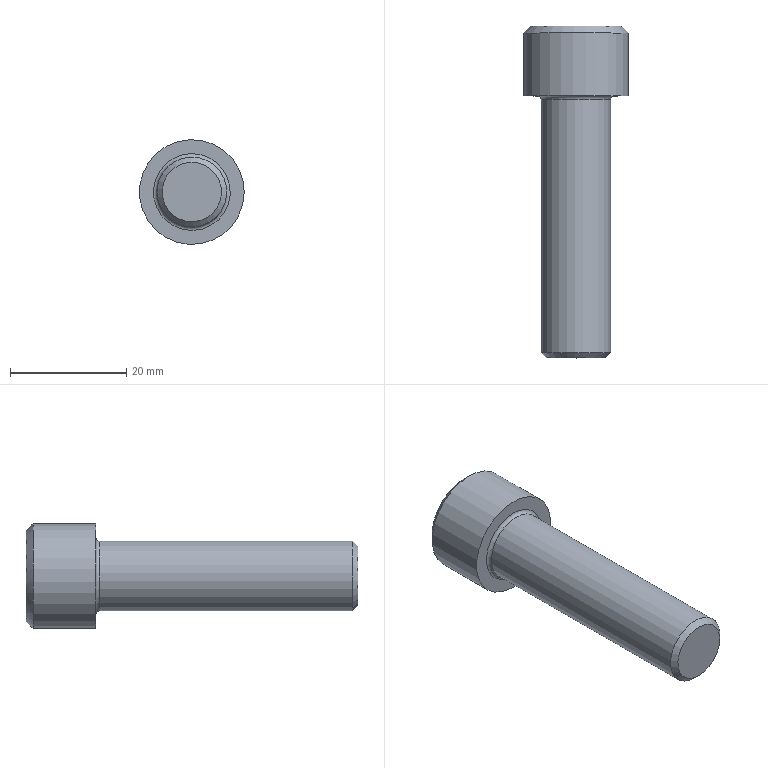Part | STEP file | solid 156 | 1 solid | 122 faces | box 18 x 57 x 18 mm | volume 7569 mm3 | plane 78 | other 29 | cylinder 6 | sphere 6 | cone 2 | torus 1 | commonest cylinder face diameters 12 x5 18 x1